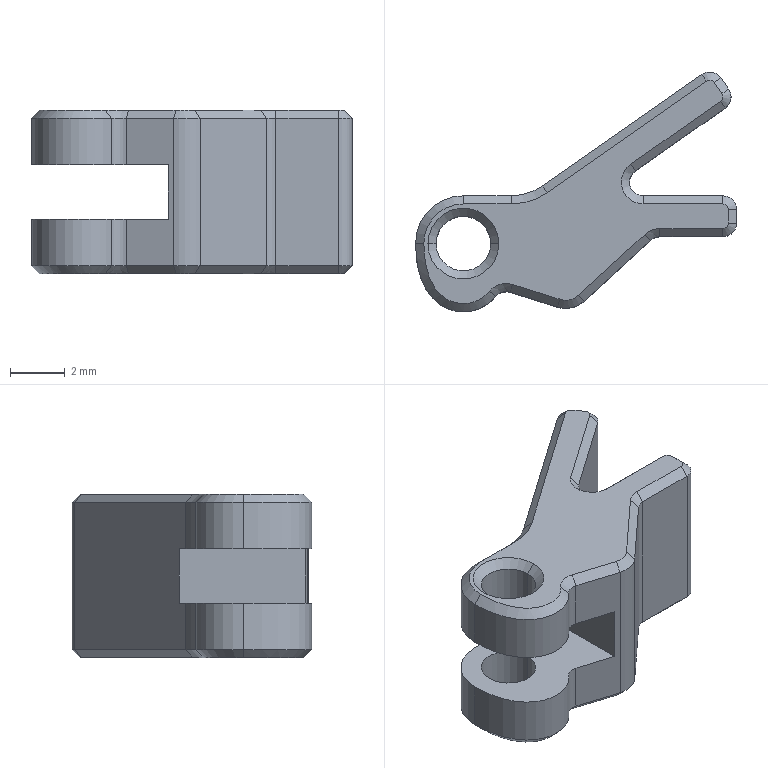Part | SolidWorks | features Attribute 3, ICE 3, Fillet 2, Chamfer 1, Extrusion 1 | 1 solid | 82 faces | box 11.75 x 8.783 x 6 mm | volume 220.036 mm3 | plane 33 | cone 26 | cylinder 19 | spline 4 | commonest cylinder face diameters 1 x10 2 x5 3.5 x2 4 x2